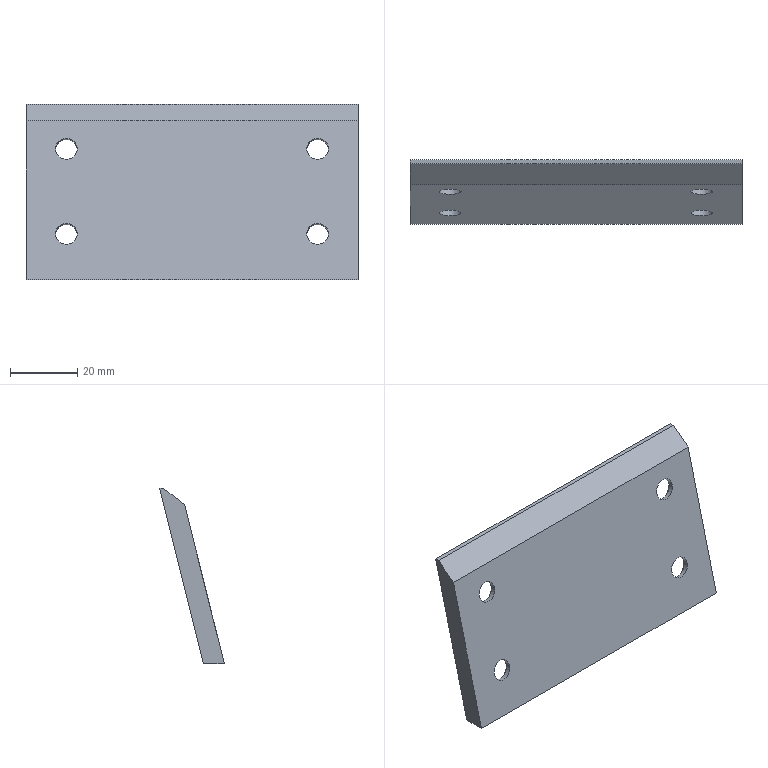Part | Creo | 1 solid | 142 faces | box 98.5 x 19.149 x 52 mm | volume 28494 mm3 | other 79 | plane 46 | cylinder 9 | cone 8 | commonest cylinder face diameters 6.4 x8 45.582 x1